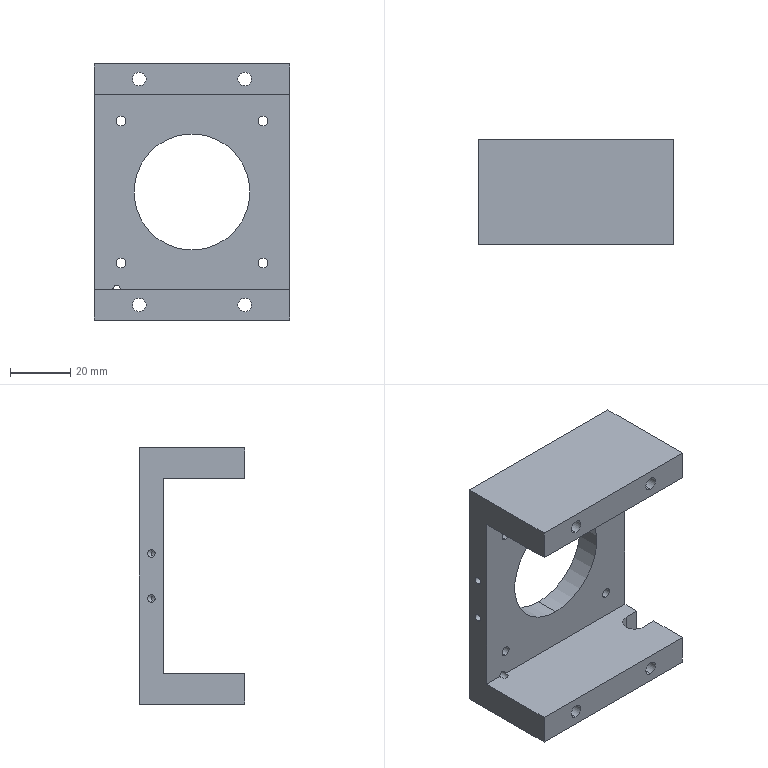Part | SolidWorks | features HoleWzd 5, ICE 3, Extrusion 1 | 1 solid | 60 faces | box 65 x 35 x 85 mm | volume 63871 mm3 | cylinder 36 | plane 17 | cone 7 | commonest cylinder face diameters 8 x10 2.5 x8 3.3 x8 4.5 x8 38.5 x2